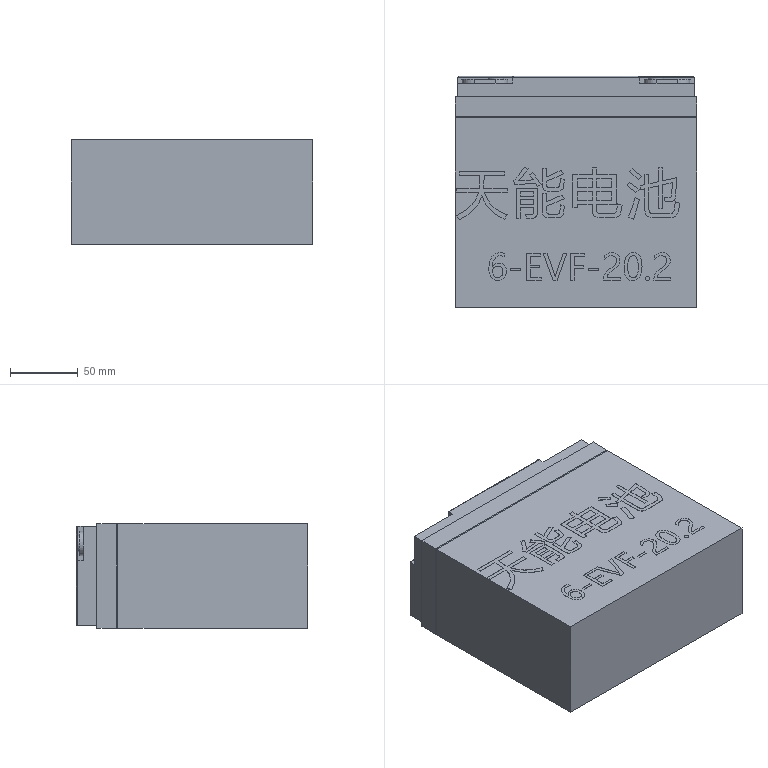Part | SolidWorks | features BaseBody 1 | 1 solid | 373 faces | box 178 x 170 x 77.1 mm | volume 2307666 mm3 | plane 232 | spline 113 | cylinder 20 | cone 4 | torus 4 | commonest cylinder face diameters 2 x8 5 x4 12 x4 18 x4